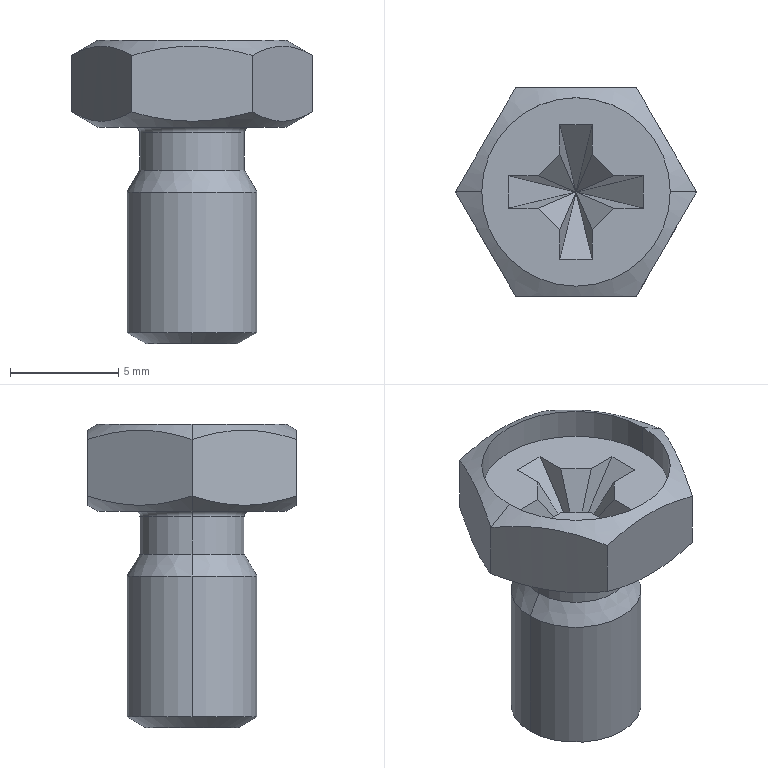Part | SolidWorks | features BaseBody 1 | 1 solid | 41 faces | box 11.131 x 9.64 x 14 mm | volume 466.025 mm3 | plane 25 | cone 8 | cylinder 6 | torus 2 | commonest cylinder face diameters 4.845 x2 6 x2 8.7 x2
STEP:
#1=CARTESIAN_POINT('',(0.,-2.134,-14.));
#2=VERTEX_POINT('',#1);
#3=CARTESIAN_POINT('',(0.,2.134,-14.));
#4=VERTEX_POINT('',#3);
#5=CARTESIAN_POINT('',(0.,0.,-14.));
#6=DIRECTION('',(0.,0.,-1.));
#7=DIRECTION('',(0.,1.,0.));
#8=AXIS2_PLACEMENT_3D('',#5,#6,#7);
#9=CIRCLE('',#8,2.134);
#10=EDGE_CURVE('',#2,#4,#9,.T.);
#11=ORIENTED_EDGE('',*,*,#10,.T.);
#12=CARTESIAN_POINT('',(0.,0.,-14.));
#13=DIRECTION('',(0.,0.,-1.));
#14=DIRECTION('',(0.,1.,0.));
#15=AXIS2_PLACEMENT_3D('',#12,#13,#14);
#16=CIRCLE('',#15,2.134);
#17=EDGE_CURVE('',#4,#2,#16,.T.);
#18=ORIENTED_EDGE('',*,*,#17,.T.);
#19=EDGE_LOOP('',(#11,#18));
#20=FACE_OUTER_BOUND('',#19,.T.);
#21=CARTESIAN_POINT('',(0.,3.,-14.));
#22=DIRECTION('',(0.,0.,1.));
#23=DIRECTION('',(1.,0.,0.));
#24=AXIS2_PLACEMENT_3D('',#21,#22,#23);
#25=PLANE('',#24);
#26=ADVANCED_FACE('',(#20),#25,.F.);
#27=CARTESIAN_POINT('',(0.,3.,-13.5));
#28=VERTEX_POINT('',#27);
#29=CARTESIAN_POINT('',(0.,3.,-13.5));
#30=DIRECTION('',(0.,0.866,0.5));
#31=VECTOR('',#30,1000.);
#32=LINE('',#29,#31);
#33=EDGE_CURVE('',#4,#28,#32,.T.);
#34=ORIENTED_EDGE('',*,*,#33,.F.);
#35=ORIENTED_EDGE('',*,*,#10,.F.);
#36=CARTESIAN_POINT('',(0.,-3.,-13.5));
#37=VERTEX_POINT('',#36);
#38=CARTESIAN_POINT('',(0.,-3.,-13.5));
#39=DIRECTION('',(0.,-0.866,0.5));
#40=VECTOR('',#39,1000.);
#41=LINE('',#38,#40);
#42=EDGE_CURVE('',#2,#37,#41,.T.);
#43=ORIENTED_EDGE('',*,*,#42,.T.);
#44=CARTESIAN_POINT('',(-3.,0.,-13.5));
#45=VERTEX_POINT('',#44);
#46=CARTESIAN_POINT('',(0.,0.,-13.5));
#47=DIRECTION('',(0.,0.,-1.));
#48=DIRECTION('',(0.,1.,0.));
#49=AXIS2_PLACEMENT_3D('',#46,#47,#48);
#50=CIRCLE('',#49,3.);
#51=EDGE_CURVE('',#37,#45,#50,.T.);
#52=ORIENTED_EDGE('',*,*,#51,.T.);
#53=CARTESIAN_POINT('',(0.,0.,-13.5));
#54=DIRECTION('',(0.,0.,-1.));
#55=DIRECTION('',(0.,1.,0.));
#56=AXIS2_PLACEMENT_3D('',#53,#54,#55);
#57=CIRCLE('',#56,3.);
#58=EDGE_CURVE('',#45,#28,#57,.T.);
#59=ORIENTED_EDGE('',*,*,#58,.T.);
#60=EDGE_LOOP('',(#34,#35,#43,#52,#59));
#61=FACE_OUTER_BOUND('',#60,.T.);
#62=CARTESIAN_POINT('',(0.,0.,-13.5));
#63=DIRECTION('',(0.,0.,1.));
#64=DIRECTION('',(0.,-1.,0.));
#65=AXIS2_PLACEMENT_3D('',#62,#63,#64);
#66=CONICAL_SURFACE('',#65,3.,1.047);
#67=ADVANCED_FACE('',(#61),#66,.T.);
#68=CARTESIAN_POINT('',(-2.673,0.,-4.));
#69=VERTEX_POINT('',#68);
#70=CARTESIAN_POINT('',(-2.423,0.,-4.25));
#71=VERTEX_POINT('',#70);
#72=CARTESIAN_POINT('',(-2.673,0.,-4.25));
#73=DIRECTION('',(0.,1.,0.));
#74=DIRECTION('',(-1.,0.,0.));
#75=AXIS2_PLACEMENT_3D('',#72,#73,#74);
#76=CIRCLE('',#75,0.25);
#77=EDGE_CURVE('',#69,#71,#76,.T.);
#78=ORIENTED_EDGE('',*,*,#77,.F.);
#79=CARTESIAN_POINT('',(2.673,0.,-4.));
#80=VERTEX_POINT('',#79);
#81=CARTESIAN_POINT('',(0.,0.,-4.));
#82=DIRECTION('',(0.,0.,1.));
#83=DIRECTION('',(1.,0.,0.));
#84=AXIS2_PLACEMENT_3D('',#81,#82,#83);
#85=CIRCLE('',#84,2.673);
#86=EDGE_CURVE('',#80,#69,#85,.T.);
#87=ORIENTED_EDGE('',*,*,#86,.F.);
#88=CARTESIAN_POINT('',(2.423,0.,-4.25));
#89=VERTEX_POINT('',#88);
#90=CARTESIAN_POINT('',(2.673,0.,-4.25));
#91=DIRECTION('',(0.,-1.,0.));
#92=DIRECTION('',(0.,0.,-1.));
#93=AXIS2_PLACEMENT_3D('',#90,#91,#92);
#94=CIRCLE('',#93,0.25);
#95=EDGE_CURVE('',#80,#89,#94,.T.);
#96=ORIENTED_EDGE('',*,*,#95,.T.);
#97=CARTESIAN_POINT('',(0.,0.,-4.25));
#98=DIRECTION('',(0.,0.,-1.));
#99=DIRECTION('',(1.,0.,0.));
#100=AXIS2_PLACEMENT_3D('',#97,#98,#99);
#101=CIRCLE('',#100,2.423);
#102=EDGE_CURVE('',#71,#89,#101,.T.);
#103=ORIENTED_EDGE('',*,*,#102,.F.);
#104=EDGE_LOOP('',(#78,#87,#96,#103));
#105=FACE_OUTER_BOUND('',#104,.T.);
#106=CARTESIAN_POINT('',(0.,0.,-4.25));
#107=DIRECTION('',(0.,0.,1.));
#108=DIRECTION('',(1.,0.,0.));
#109=AXIS2_PLACEMENT_3D('',#106,#107,#108);
#110=TOROIDAL_SURFACE('',#109,2.673,0.25);
#111=ADVANCED_FACE('',(#105),#110,.F.);
#112=CARTESIAN_POINT('',(-0.75,-1.75,-1.4));
#113=VERTEX_POINT('',#112);
#114=CARTESIAN_POINT('',(0.,0.,-4.26));
#115=VERTEX_POINT('',#114);
#116=CARTESIAN_POINT('',(-0.75,-1.75,-1.4));
#117=DIRECTION('',(0.2183,0.5093,-0.8324));
#118=VECTOR('',#117,1000.);
#119=LINE('',#116,#118);
#120=EDGE_CURVE('',#113,#115,#119,.T.);
#121=ORIENTED_EDGE('',*,*,#120,.F.);
#122=CARTESIAN_POINT('',(-0.75,-3.1,-1.4));
#123=VERTEX_POINT('',#122);
#124=CARTESIAN_POINT('',(-0.75,-1.75,-1.4));
#125=DIRECTION('',(0.,-1.,0.));
#126=VECTOR('',#125,1000.);
#127=LINE('',#124,#126);
#128=EDGE_CURVE('',#113,#123,#127,.T.);
#129=ORIENTED_EDGE('',*,*,#128,.T.);
#130=CARTESIAN_POINT('',(-0.75,-3.1,-1.4));
#131=DIRECTION('',(0.1751,0.7236,-0.6676));
#132=VECTOR('',#131,1000.);
#133=LINE('',#130,#132);
#134=EDGE_CURVE('',#123,#115,#133,.T.);
#135=ORIENTED_EDGE('',*,*,#134,.T.);
#136=EDGE_LOOP('',(#121,#129,#135));
#137=FACE_OUTER_BOUND('',#136,.T.);
#138=CARTESIAN_POINT('',(-0.75,-1.75,-1.4));
#139=DIRECTION('',(-0.9673,0.,-0.2537));
#140=DIRECTION('',(-0.2537,0.,0.9673));
#141=AXIS2_PLACEMENT_3D('',#138,#139,#140);
#142=PLANE('',#141);
#143=ADVANCED_FACE('',(#137),#142,.F.);
#144=ORIENTED_EDGE('',*,*,#134,.F.);
#145=CARTESIAN_POINT('',(0.75,-3.1,-1.4));
#146=VERTEX_POINT('',#145);
#147=CARTESIAN_POINT('',(-0.75,-3.1,-1.4));
#148=DIRECTION('',(1.,0.,0.));
#149=VECTOR('',#148,1000.);
#150=LINE('',#147,#149);
#151=EDGE_CURVE('',#123,#146,#150,.T.);
#152=ORIENTED_EDGE('',*,*,#151,.T.);
#153=CARTESIAN_POINT('',(0.75,-3.1,-1.4));
#154=DIRECTION('',(-0.1751,0.7236,-0.6676));
#155=VECTOR('',#154,1000.);
#156=LINE('',#153,#155);
#157=EDGE_CURVE('',#146,#115,#156,.T.);
#158=ORIENTED_EDGE('',*,*,#157,.T.);
#159=EDGE_LOOP('',(#144,#152,#158));
#160=FACE_OUTER_BOUND('',#159,.T.);
#161=CARTESIAN_POINT('',(-0.75,-3.1,-1.4));
#162=DIRECTION('',(0.,-0.6781,-0.735));
#163=DIRECTION('',(0.,-0.735,0.6781));
#164=AXIS2_PLACEMENT_3D('',#161,#162,#163);
#165=PLANE('',#164);
#166=ADVANCED_FACE('',(#160),#165,.F.);
#167=CARTESIAN_POINT('',(-1.75,-0.75,-1.4));
#168=VERTEX_POINT('',#167);
#169=CARTESIAN_POINT('',(-1.75,-0.75,-1.4));
#170=DIRECTION('',(0.5093,0.2183,-0.8324));
#171=VECTOR('',#170,1000.);
#172=LINE('',#169,#171);
#173=EDGE_CURVE('',#168,#115,#172,.T.);
#174=ORIENTED_EDGE('',*,*,#173,.F.);
#175=CARTESIAN_POINT('',(-1.75,-0.75,-1.4));
#176=DIRECTION('',(0.7071,-0.7071,0.));
#177=VECTOR('',#176,1000.);
#178=LINE('',#175,#177);
#179=EDGE_CURVE('',#168,#113,#178,.T.);
#180=ORIENTED_EDGE('',*,*,#179,.T.);
#181=ORIENTED_EDGE('',*,*,#120,.T.);
#182=EDGE_LOOP('',(#174,#180,#181));
#183=FACE_OUTER_BOUND('',#182,.T.);
#184=CARTESIAN_POINT('',(-1.75,-0.75,-1.4));
#185=DIRECTION('',(-0.6015,-0.6015,-0.5258));
#186=DIRECTION('',(-0.7071,0.7071,0.));
#187=AXIS2_PLACEMENT_3D('',#184,#185,#186);
#188=PLANE('',#187);
#189=ADVANCED_FACE('',(#183),#188,.F.);
#190=ORIENTED_EDGE('',*,*,#157,.F.);
#191=CARTESIAN_POINT('',(0.75,-1.75,-1.4));
#192=VERTEX_POINT('',#191);
#193=CARTESIAN_POINT('',(0.75,-1.75,-1.4));
#194=DIRECTION('',(0.,1.,0.));
#195=VECTOR('',#194,1000.);
#196=LINE('',#193,#195);
#197=EDGE_CURVE('',#146,#192,#196,.T.);
#198=ORIENTED_EDGE('',*,*,#197,.T.);
#199=CARTESIAN_POINT('',(0.75,-1.75,-1.4));
#200=DIRECTION('',(-0.2183,0.5093,-0.8324));
#201=VECTOR('',#200,1000.);
#202=LINE('',#199,#201);
#203=EDGE_CURVE('',#192,#115,#202,.T.);
#204=ORIENTED_EDGE('',*,*,#203,.T.);
#205=EDGE_LOOP('',(#190,#198,#204));
#206=FACE_OUTER_BOUND('',#205,.T.);
#207=CARTESIAN_POINT('',(0.75,-3.1,-1.4));
#208=DIRECTION('',(0.9673,0.,-0.2537));
#209=DIRECTION('',(0.,-1.,0.));
#210=AXIS2_PLACEMENT_3D('',#207,#208,#209);
#211=PLANE('',#210);
#212=ADVANCED_FACE('',(#206),#211,.F.);
#213=CARTESIAN_POINT('',(-3.1,-0.75,-1.4));
#214=VERTEX_POINT('',#213);
#215=CARTESIAN_POINT('',(-3.1,-0.75,-1.4));
#216=DIRECTION('',(0.7236,0.1751,-0.6676));
#217=VECTOR('',#216,1000.);
#218=LINE('',#215,#217);
#219=EDGE_CURVE('',#214,#115,#218,.T.);
#220=ORIENTED_EDGE('',*,*,#219,.F.);
#221=CARTESIAN_POINT('',(-3.1,-0.75,-1.4));
#222=DIRECTION('',(1.,0.,0.));
#223=VECTOR('',#222,1000.);
#224=LINE('',#221,#223);
#225=EDGE_CURVE('',#214,#168,#224,.T.);
#226=ORIENTED_EDGE('',*,*,#225,.T.);
#227=ORIENTED_EDGE('',*,*,#173,.T.);
#228=EDGE_LOOP('',(#220,#226,#227));
#229=FACE_OUTER_BOUND('',#228,.T.);
#230=CARTESIAN_POINT('',(-3.1,-0.75,-1.4));
#231=DIRECTION('',(0.,-0.9673,-0.2537));
#232=DIRECTION('',(0.,0.2537,-0.9673));
#233=AXIS2_PLACEMENT_3D('',#230,#231,#232);
#234=PLANE('',#233);
#235=ADVANCED_FACE('',(#229),#234,.F.);
#236=ORIENTED_EDGE('',*,*,#203,.F.);
#237=CARTESIAN_POINT('',(1.75,-0.75,-1.4));
#238=VERTEX_POINT('',#237);
#239=CARTESIAN_POINT('',(1.75,-0.75,-1.4));
#240=DIRECTION('',(0.7071,0.7071,0.));
#241=VECTOR('',#240,1000.);
#242=LINE('',#239,#241);
#243=EDGE_CURVE('',#192,#238,#242,.T.);
#244=ORIENTED_EDGE('',*,*,#243,.T.);
#245=CARTESIAN_POINT('',(1.75,-0.75,-1.4));
#246=DIRECTION('',(-0.5093,0.2183,-0.8324));
#247=VECTOR('',#246,1000.);
#248=LINE('',#245,#247);
#249=EDGE_CURVE('',#238,#115,#248,.T.);
#250=ORIENTED_EDGE('',*,*,#249,.T.);
#251=EDGE_LOOP('',(#236,#244,#250));
#252=FACE_OUTER_BOUND('',#251,.T.);
#253=CARTESIAN_POINT('',(0.75,-1.75,-1.4));
#254=DIRECTION('',(0.6015,-0.6015,-0.5258));
#255=DIRECTION('',(0.,0.6581,-0.7529));
#256=AXIS2_PLACEMENT_3D('',#253,#254,#255);
#257=PLANE('',#256);
#258=ADVANCED_FACE('',(#252),#257,.F.);
#259=CARTESIAN_POINT('',(-3.1,0.75,-1.4));
#260=VERTEX_POINT('',#259);
#261=CARTESIAN_POINT('',(-3.1,0.75,-1.4));
#262=DIRECTION('',(0.7236,-0.1751,-0.6676));
#263=VECTOR('',#262,1000.);
#264=LINE('',#261,#263);
#265=EDGE_CURVE('',#260,#115,#264,.T.);
#266=ORIENTED_EDGE('',*,*,#265,.F.);
#267=CARTESIAN_POINT('',(-3.1,0.75,-1.4));
#268=DIRECTION('',(0.,-1.,0.));
#269=VECTOR('',#268,1000.);
#270=LINE('',#267,#269);
#271=EDGE_CURVE('',#260,#214,#270,.T.);
#272=ORIENTED_EDGE('',*,*,#271,.T.);
#273=ORIENTED_EDGE('',*,*,#219,.T.);
#274=EDGE_LOOP('',(#266,#272,#273));
#275=FACE_OUTER_BOUND('',#274,.T.);
#276=CARTESIAN_POINT('',(-3.1,0.75,-1.4));
#277=DIRECTION('',(-0.6781,0.,-0.735));
#278=DIRECTION('',(-0.735,0.,0.6781));
#279=AXIS2_PLACEMENT_3D('',#276,#277,#278);
#280=PLANE('',#279);
#281=ADVANCED_FACE('',(#275),#280,.F.);
#282=ORIENTED_EDGE('',*,*,#249,.F.);
#283=CARTESIAN_POINT('',(3.1,-0.75,-1.4));
#284=VERTEX_POINT('',#283);
#285=CARTESIAN_POINT('',(1.75,-0.75,-1.4));
#286=DIRECTION('',(1.,0.,0.));
#287=VECTOR('',#286,1000.);
#288=LINE('',#285,#287);
#289=EDGE_CURVE('',#238,#284,#288,.T.);
#290=ORIENTED_EDGE('',*,*,#289,.T.);
#291=CARTESIAN_POINT('',(3.1,-0.75,-1.4));
#292=DIRECTION('',(-0.7236,0.1751,-0.6676));
#293=VECTOR('',#292,1000.);
#294=LINE('',#291,#293);
#295=EDGE_CURVE('',#284,#115,#294,.T.);
#296=ORIENTED_EDGE('',*,*,#295,.T.);
#297=EDGE_LOOP('',(#282,#290,#296));
#298=FACE_OUTER_BOUND('',#297,.T.);
#299=CARTESIAN_POINT('',(1.75,-0.75,-1.4));
#300=DIRECTION('',(0.,-0.9673,-0.2537));
#301=DIRECTION('',(0.,0.2537,-0.9673));
#302=AXIS2_PLACEMENT_3D('',#299,#300,#301);
#303=PLANE('',#302);
#304=ADVANCED_FACE('',(#298),#303,.F.);
#305=CARTESIAN_POINT('',(-1.75,0.75,-1.4));
#306=VERTEX_POINT('',#305);
#307=CARTESIAN_POINT('',(-1.75,0.75,-1.4));
#308=DIRECTION('',(0.5093,-0.2183,-0.8324));
#309=VECTOR('',#308,1000.);
#310=LINE('',#307,#309);
#311=EDGE_CURVE('',#306,#115,#310,.T.);
#312=ORIENTED_EDGE('',*,*,#311,.F.);
#313=CARTESIAN_POINT('',(-3.1,0.75,-1.4));
#314=DIRECTION('',(-1.,0.,0.));
#315=VECTOR('',#314,1000.);
#316=LINE('',#313,#315);
#317=EDGE_CURVE('',#306,#260,#316,.T.);
#318=ORIENTED_EDGE('',*,*,#317,.T.);
#319=ORIENTED_EDGE('',*,*,#265,.T.);
#320=EDGE_LOOP('',(#312,#318,#319));
#321=FACE_OUTER_BOUND('',#320,.T.);
#322=CARTESIAN_POINT('',(-1.75,0.75,-1.4));
#323=DIRECTION('',(0.,0.9673,-0.2537));
#324=DIRECTION('',(-1.,0.,0.));
#325=AXIS2_PLACEMENT_3D('',#322,#323,#324);
#326=PLANE('',#325);
#327=ADVANCED_FACE('',(#321),#326,.F.);
#328=ORIENTED_EDGE('',*,*,#295,.F.);
#329=CARTESIAN_POINT('',(3.1,0.75,-1.4));
#330=VERTEX_POINT('',#329);
#331=CARTESIAN_POINT('',(3.1,0.75,-1.4));
#332=DIRECTION('',(0.,1.,0.));
#333=VECTOR('',#332,1000.);
#334=LINE('',#331,#333);
#335=EDGE_CURVE('',#284,#330,#334,.T.);
#336=ORIENTED_EDGE('',*,*,#335,.T.);
#337=CARTESIAN_POINT('',(3.1,0.75,-1.4));
#338=DIRECTION('',(-0.7236,-0.1751,-0.6676));
#339=VECTOR('',#338,1000.);
#340=LINE('',#337,#339);
#341=EDGE_CURVE('',#330,#115,#340,.T.);
#342=ORIENTED_EDGE('',*,*,#341,.T.);
#343=EDGE_LOOP('',(#328,#336,#342));
#344=FACE_OUTER_BOUND('',#343,.T.);
#345=CARTESIAN_POINT('',(3.1,-0.75,-1.4));
#346=DIRECTION('',(0.6781,0.,-0.735));
#347=DIRECTION('',(0.,-1.,0.));
#348=AXIS2_PLACEMENT_3D('',#345,#346,#347);
#349=PLANE('',#348);
#350=ADVANCED_FACE('',(#344),#349,.F.);
#351=CARTESIAN_POINT('',(-0.75,1.75,-1.4));
#352=VERTEX_POINT('',#351);
#353=CARTESIAN_POINT('',(-0.75,1.75,-1.4));
#354=DIRECTION('',(0.2183,-0.5093,-0.8324));
#355=VECTOR('',#354,1000.);
#356=LINE('',#353,#355);
#357=EDGE_CURVE('',#352,#115,#356,.T.);
#358=ORIENTED_EDGE('',*,*,#357,.F.);
#359=CARTESIAN_POINT('',(-0.75,1.75,-1.4));
#360=DIRECTION('',(-0.7071,-0.7071,0.));
#361=VECTOR('',#360,1000.);
#362=LINE('',#359,#361);
#363=EDGE_CURVE('',#352,#306,#362,.T.);
#364=ORIENTED_EDGE('',*,*,#363,.T.);
#365=ORIENTED_EDGE('',*,*,#311,.T.);
#366=EDGE_LOOP('',(#358,#364,#365));
#367=FACE_OUTER_BOUND('',#366,.T.);
#368=CARTESIAN_POINT('',(-0.75,1.75,-1.4));
#369=DIRECTION('',(-0.6015,0.6015,-0.5258));
#370=DIRECTION('',(-0.6581,0.,0.7529));
#371=AXIS2_PLACEMENT_3D('',#368,#369,#370);
#372=PLANE('',#371);
#373=ADVANCED_FACE('',(#367),#372,.F.);
#374=ORIENTED_EDGE('',*,*,#341,.F.);
#375=CARTESIAN_POINT('',(1.75,0.75,-1.4));
#376=VERTEX_POINT('',#375);
#377=CARTESIAN_POINT('',(1.75,0.75,-1.4));
#378=DIRECTION('',(-1.,0.,0.));
#379=VECTOR('',#378,1000.);
#380=LINE('',#377,#379);
#381=EDGE_CURVE('',#330,#376,#380,.T.);
#382=ORIENTED_EDGE('',*,*,#381,.T.);
#383=CARTESIAN_POINT('',(1.75,0.75,-1.4));
#384=DIRECTION('',(-0.5093,-0.2183,-0.8324));
#385=VECTOR('',#384,1000.);
#386=LINE('',#383,#385);
#387=EDGE_CURVE('',#376,#115,#386,.T.);
#388=ORIENTED_EDGE('',*,*,#387,.T.);
#389=EDGE_LOOP('',(#374,#382,#388));
#390=FACE_OUTER_BOUND('',#389,.T.);
#391=CARTESIAN_POINT('',(3.1,0.75,-1.4));
#392=DIRECTION('',(0.,0.9673,-0.2537));
#393=DIRECTION('',(-1.,0.,0.));
#394=AXIS2_PLACEMENT_3D('',#391,#392,#393);
#395=PLANE('',#394);
#396=ADVANCED_FACE('',(#390),#395,.F.);
#397=CARTESIAN_POINT('',(-0.75,3.1,-1.4));
#398=VERTEX_POINT('',#397);
#399=CARTESIAN_POINT('',(-0.75,3.1,-1.4));
#400=DIRECTION('',(0.1751,-0.7236,-0.6676));
#401=VECTOR('',#400,1000.);
#402=LINE('',#399,#401);
#403=EDGE_CURVE('',#398,#115,#402,.T.);
#404=ORIENTED_EDGE('',*,*,#403,.F.);
#405=CARTESIAN_POINT('',(-0.75,3.1,-1.4));
#406=DIRECTION('',(0.,-1.,0.));
#407=VECTOR('',#406,1000.);
#408=LINE('',#405,#407);
#409=EDGE_CURVE('',#398,#352,#408,.T.);
#410=ORIENTED_EDGE('',*,*,#409,.T.);
#411=ORIENTED_EDGE('',*,*,#357,.T.);
#412=EDGE_LOOP('',(#404,#410,#411));
#413=FACE_OUTER_BOUND('',#412,.T.);
#414=CARTESIAN_POINT('',(-0.75,3.1,-1.4));
#415=DIRECTION('',(-0.9673,0.,-0.2537));
#416=DIRECTION('',(-0.2537,0.,0.9673));
#417=AXIS2_PLACEMENT_3D('',#414,#415,#416);
#418=PLANE('',#417);
#419=ADVANCED_FACE('',(#413),#418,.F.);
#420=ORIENTED_EDGE('',*,*,#387,.F.);
#421=CARTESIAN_POINT('',(0.75,1.75,-1.4));
#422=VERTEX_POINT('',#421);
#423=CARTESIAN_POINT('',(0.75,1.75,-1.4));
#424=DIRECTION('',(-0.7071,0.7071,0.));
#425=VECTOR('',#424,1000.);
#426=LINE('',#423,#425);
#427=EDGE_CURVE('',#376,#422,#426,.T.);
#428=ORIENTED_EDGE('',*,*,#427,.T.);
#429=CARTESIAN_POINT('',(0.75,1.75,-1.4));
#430=DIRECTION('',(-0.2183,-0.5093,-0.8324));
#431=VECTOR('',#430,1000.);
#432=LINE('',#429,#431);
#433=EDGE_CURVE('',#422,#115,#432,.T.);
#434=ORIENTED_EDGE('',*,*,#433,.T.);
#435=EDGE_LOOP('',(#420,#428,#434));
#436=FACE_OUTER_BOUND('',#435,.T.);
#437=CARTESIAN_POINT('',(1.75,0.75,-1.4));
#438=DIRECTION('',(0.6015,0.6015,-0.5258));
#439=DIRECTION('',(0.,-0.6581,-0.7529));
#440=AXIS2_PLACEMENT_3D('',#437,#438,#439);
#441=PLANE('',#440);
#442=ADVANCED_FACE('',(#436),#441,.F.);
#443=CARTESIAN_POINT('',(0.75,3.1,-1.4));
#444=VERTEX_POINT('',#443);
#445=CARTESIAN_POINT('',(0.75,3.1,-1.4));
#446=DIRECTION('',(-0.1751,-0.7236,-0.6676));
#447=VECTOR('',#446,1000.);
#448=LINE('',#445,#447);
#449=EDGE_CURVE('',#444,#115,#448,.T.);
#450=ORIENTED_EDGE('',*,*,#449,.F.);
#451=CARTESIAN_POINT('',(-0.75,3.1,-1.4));
#452=DIRECTION('',(-1.,0.,0.));
#453=VECTOR('',#452,1000.);
#454=LINE('',#451,#453);
#455=EDGE_CURVE('',#444,#398,#454,.T.);
#456=ORIENTED_EDGE('',*,*,#455,.T.);
#457=ORIENTED_EDGE('',*,*,#403,.T.);
#458=EDGE_LOOP('',(#450,#456,#457));
#459=FACE_OUTER_BOUND('',#458,.T.);
#460=CARTESIAN_POINT('',(0.75,3.1,-1.4));
#461=DIRECTION('',(0.,0.6781,-0.735));
#462=DIRECTION('',(-1.,0.,0.));
#463=AXIS2_PLACEMENT_3D('',#460,#461,#462);
#464=PLANE('',#463);
#465=ADVANCED_FACE('',(#459),#464,.F.);
#466=ORIENTED_EDGE('',*,*,#433,.F.);
#467=CARTESIAN_POINT('',(0.75,3.1,-1.4));
#468=DIRECTION('',(0.,1.,0.));
#469=VECTOR('',#468,1000.);
#470=LINE('',#467,#469);
#471=EDGE_CURVE('',#422,#444,#470,.T.);
#472=ORIENTED_EDGE('',*,*,#471,.T.);
#473=ORIENTED_EDGE('',*,*,#449,.T.);
#474=EDGE_LOOP('',(#466,#472,#473));
#475=FACE_OUTER_BOUND('',#474,.T.);
#476=CARTESIAN_POINT('',(0.75,1.75,-1.4));
#477=DIRECTION('',(0.9673,0.,-0.2537));
#478=DIRECTION('',(0.,-1.,0.));
#479=AXIS2_PLACEMENT_3D('',#476,#477,#478);
#480=PLANE('',#479);
#481=ADVANCED_FACE('',(#475),#480,.F.);
#482=ORIENTED_EDGE('',*,*,#471,.F.);
#483=ORIENTED_EDGE('',*,*,#427,.F.);
#484=ORIENTED_EDGE('',*,*,#381,.F.);
#485=ORIENTED_EDGE('',*,*,#335,.F.);
#486=ORIENTED_EDGE('',*,*,#289,.F.);
#487=ORIENTED_EDGE('',*,*,#243,.F.);
#488=ORIENTED_EDGE('',*,*,#197,.F.);
#489=ORIENTED_EDGE('',*,*,#151,.F.);
#490=ORIENTED_EDGE('',*,*,#128,.F.);
#491=ORIENTED_EDGE('',*,*,#179,.F.);
#492=ORIENTED_EDGE('',*,*,#225,.F.);
#493=ORIENTED_EDGE('',*,*,#271,.F.);
#494=ORIENTED_EDGE('',*,*,#317,.F.);
#495=ORIENTED_EDGE('',*,*,#363,.F.);
#496=ORIENTED_EDGE('',*,*,#409,.F.);
#497=ORIENTED_EDGE('',*,*,#455,.F.);
#498=EDGE_LOOP('',(#482,#483,#484,#485,#486,#487,#488,#489,#490,#491,#492,#493,#494,#495,#496,#497));
#499=FACE_BOUND('',#498,.T.);
#500=CARTESIAN_POINT('',(4.35,0.,-1.4));
#501=VERTEX_POINT('',#500);
#502=CARTESIAN_POINT('',(-4.35,0.,-1.4));
#503=VERTEX_POINT('',#502);
#504=CARTESIAN_POINT('',(0.,0.,-1.4));
#505=DIRECTION('',(0.,0.,1.));
#506=DIRECTION('',(1.,0.,0.));
#507=AXIS2_PLACEMENT_3D('',#504,#505,#506);
#508=CIRCLE('',#507,4.35);
#509=EDGE_CURVE('',#501,#503,#508,.T.);
#510=ORIENTED_EDGE('',*,*,#509,.T.);
#511=CARTESIAN_POINT('',(0.,0.,-1.4));
#512=DIRECTION('',(0.,0.,1.));
#513=DIRECTION('',(1.,0.,0.));
#514=AXIS2_PLACEMENT_3D('',#511,#512,#513);
#515=CIRCLE('',#514,4.35);
#516=EDGE_CURVE('',#503,#501,#515,.T.);
#517=ORIENTED_EDGE('',*,*,#516,.T.);
#518=EDGE_LOOP('',(#510,#517));
#519=FACE_OUTER_BOUND('',#518,.T.);
#520=CARTESIAN_POINT('',(0.,0.,-1.4));
#521=DIRECTION('',(0.,0.,1.));
#522=DIRECTION('',(1.,0.,0.));
#523=AXIS2_PLACEMENT_3D('',#520,#521,#522);
#524=PLANE('',#523);
#525=ADVANCED_FACE('',(#499,#519),#524,.T.);
#526=CARTESIAN_POINT('',(-4.35,0.,0.));
#527=VERTEX_POINT('',#526);
#528=CARTESIAN_POINT('',(-4.35,0.,-1.4));
#529=DIRECTION('',(0.,0.,1.));
#530=VECTOR('',#529,1000.);
#531=LINE('',#528,#530);
#532=EDGE_CURVE('',#503,#527,#531,.T.);
#533=ORIENTED_EDGE('',*,*,#532,.F.);
#534=ORIENTED_EDGE('',*,*,#509,.F.);
#535=CARTESIAN_POINT('',(4.35,0.,0.));
#536=VERTEX_POINT('',#535);
#537=CARTESIAN_POINT('',(4.35,0.,-1.4));
#538=DIRECTION('',(0.,0.,1.));
#539=VECTOR('',#538,1000.);
#540=LINE('',#537,#539);
#541=EDGE_CURVE('',#501,#536,#540,.T.);
#542=ORIENTED_EDGE('',*,*,#541,.T.);
#543=CARTESIAN_POINT('',(0.,0.,0.));
#544=DIRECTION('',(0.,0.,1.));
#545=DIRECTION('',(1.,0.,0.));
#546=AXIS2_PLACEMENT_3D('',#543,#544,#545);
#547=CIRCLE('',#546,4.35);
#548=EDGE_CURVE('',#536,#527,#547,.T.);
#549=ORIENTED_EDGE('',*,*,#548,.T.);
#550=EDGE_LOOP('',(#533,#534,#542,#549));
#551=FACE_OUTER_BOUND('',#550,.T.);
#552=CARTESIAN_POINT('',(0.,0.,-1.4));
#553=DIRECTION('',(0.,0.,1.));
#554=DIRECTION('',(1.,0.,0.));
#555=AXIS2_PLACEMENT_3D('',#552,#553,#554);
#556=CYLINDRICAL_SURFACE('',#555,4.35);
#557=ADVANCED_FACE('',(#551),#556,.F.);
#558=CARTESIAN_POINT('',(5.566,0.,-0.7019));
#559=VERTEX_POINT('',#558);
#560=CARTESIAN_POINT('',(4.35,0.,0.));
#561=DIRECTION('',(0.866,0.,-0.5));
#562=VECTOR('',#561,1000.);
#563=LINE('',#560,#562);
#564=EDGE_CURVE('',#536,#559,#563,.T.);
#565=ORIENTED_EDGE('',*,*,#564,.F.);
#566=CARTESIAN_POINT('',(0.,0.,0.));
#567=DIRECTION('',(0.,0.,1.));
#568=DIRECTION('',(1.,0.,0.));
#569=AXIS2_PLACEMENT_3D('',#566,#567,#568);
#570=CIRCLE('',#569,4.35);
#571=EDGE_CURVE('',#527,#536,#570,.T.);
#572=ORIENTED_EDGE('',*,*,#571,.F.);
#573=CARTESIAN_POINT('',(-5.566,0.,-0.7019));
#574=VERTEX_POINT('',#573);
#575=CARTESIAN_POINT('',(-4.35,0.,0.));
#576=DIRECTION('',(-0.866,0.,-0.5));
#577=VECTOR('',#576,1000.);
#578=LINE('',#575,#577);
#579=EDGE_CURVE('',#527,#574,#578,.T.);
#580=ORIENTED_EDGE('',*,*,#579,.T.);
#581=CARTESIAN_POINT('',(-2.783,-4.82,-0.7019));
#582=VERTEX_POINT('',#581);
#583=CARTESIAN_POINT('',(-5.566,0.,-0.7019));
#584=CARTESIAN_POINT('',(-5.447,-0.2048,-0.6336));
#585=CARTESIAN_POINT('',(-5.332,-0.4051,-0.5733));
#586=CARTESIAN_POINT('',(-5.161,-0.7017,-0.4948));
#587=CARTESIAN_POINT('',(-5.104,-0.7999,-0.4706));
#588=CARTESIAN_POINT('',(-5.019,-0.9467,-0.4374));
#589=CARTESIAN_POINT('',(-4.977,-1.02,-0.4215));
#590=CARTESIAN_POINT('',(-4.935,-1.093,-0.4067));
#591=CARTESIAN_POINT('',(-4.907,-1.142,-0.3971));
#592=CARTESIAN_POINT('',(-4.894,-1.165,-0.3927));
#593=CARTESIAN_POINT('',(-4.759,-1.398,-0.3492));
#594=CARTESIAN_POINT('',(-4.642,-1.6,-0.3201));
#595=CARTESIAN_POINT('',(-4.41,-2.002,-0.2813));
#596=CARTESIAN_POINT('',(-4.295,-2.201,-0.2715));
#597=CARTESIAN_POINT('',(-4.059,-2.61,-0.2712));
#598=CARTESIAN_POINT('',(-3.942,-2.811,-0.2808));
#599=CARTESIAN_POINT('',(-3.767,-3.115,-0.3097));
#600=CARTESIAN_POINT('',(-3.709,-3.216,-0.3218));
#601=CARTESIAN_POINT('',(-3.62,-3.369,-0.3436));
#602=CARTESIAN_POINT('',(-3.576,-3.446,-0.3554));
#603=CARTESIAN_POINT('',(-3.532,-3.523,-0.3685));
#604=CARTESIAN_POINT('',(-3.502,-3.575,-0.3776));
#605=CARTESIAN_POINT('',(-3.486,-3.602,-0.3826));
#606=CARTESIAN_POINT('',(-3.247,-4.017,-0.4599));
#607=CARTESIAN_POINT('',(-3.02,-4.409,-0.5648));
#608=CARTESIAN_POINT('',(-2.783,-4.82,-0.7019));
#609=B_SPLINE_CURVE_WITH_KNOTS('',3,(#583,#584,#585,#586,#587,#588,#589,#590,#591,#592,#593,#594,#595,#596,#597,#598,#599,#600,#601,#602,#603,#604,#605,#606,#607,#608),.UNSPECIFIED.,.F.,.F.,(4,2,2,1,2,2,2,2,2,2,1,2,2,4),(0.,0.125,0.1875,0.2187,0.2344,0.25,0.375,0.5,0.625,0.6875,0.7188,0.7344,0.75,1.),.UNSPECIFIED.);
#610=EDGE_CURVE('',#574,#582,#609,.T.);
#611=ORIENTED_EDGE('',*,*,#610,.T.);
#612=CARTESIAN_POINT('',(2.783,-4.82,-0.7019));
#613=VERTEX_POINT('',#612);
#614=CARTESIAN_POINT('',(-2.783,-4.82,-0.7019));
#615=CARTESIAN_POINT('',(-2.545,-4.82,-0.6332));
#616=CARTESIAN_POINT('',(-2.312,-4.82,-0.5726));
#617=CARTESIAN_POINT('',(-1.968,-4.82,-0.4938));
#618=CARTESIAN_POINT('',(-1.854,-4.82,-0.4695));
#619=CARTESIAN_POINT('',(-1.684,-4.82,-0.4362));
#620=CARTESIAN_POINT('',(-1.599,-4.82,-0.4202));
#621=CARTESIAN_POINT('',(-1.515,-4.82,-0.4055));
#622=CARTESIAN_POINT('',(-1.458,-4.82,-0.3959));
#623=CARTESIAN_POINT('',(-1.431,-4.82,-0.3914));
#624=CARTESIAN_POINT('',(-0.9247,-4.82,-0.3097));
#625=CARTESIAN_POINT('',(-0.4706,-4.82,-0.2713));
#626=CARTESIAN_POINT('',(0.1187,-4.82,-0.2714));
#627=CARTESIAN_POINT('',(0.2362,-4.82,-0.2739));
#628=CARTESIAN_POINT('',(0.4717,-4.82,-0.2839));
#629=CARTESIAN_POINT('',(0.5915,-4.82,-0.2915));
#630=CARTESIAN_POINT('',(0.826,-4.82,-0.3112));
#631=CARTESIAN_POINT('',(0.9429,-4.82,-0.3234));
#632=CARTESIAN_POINT('',(1.119,-4.82,-0.3451));
#633=CARTESIAN_POINT('',(1.206,-4.82,-0.3569));
#634=CARTESIAN_POINT('',(1.295,-4.82,-0.3699));
#635=CARTESIAN_POINT('',(1.354,-4.82,-0.3789));
#636=CARTESIAN_POINT('',(1.385,-4.82,-0.3838));
#637=CARTESIAN_POINT('',(1.86,-4.82,-0.4611));
#638=CARTESIAN_POINT('',(2.311,-4.82,-0.5656));
#639=CARTESIAN_POINT('',(2.783,-4.82,-0.7019));
#640=B_SPLINE_CURVE_WITH_KNOTS('',3,(#614,#615,#616,#617,#618,#619,#620,#621,#622,#623,#624,#625,#626,#627,#628,#629,#630,#631,#632,#633,#634,#635,#636,#637,#638,#639),.UNSPECIFIED.,.F.,.F.,(4,2,2,1,2,2,2,2,2,2,1,2,2,4),(0.,0.125,0.1875,0.2188,0.2344,0.25,0.5,0.5625,0.625,0.6875,0.7188,0.7344,0.75,1.),.UNSPECIFIED.);
#641=EDGE_CURVE('',#582,#613,#640,.T.);
#642=ORIENTED_EDGE('',*,*,#641,.T.);
#643=CARTESIAN_POINT('',(2.783,-4.82,-0.7019));
#644=CARTESIAN_POINT('',(2.901,-4.615,-0.6336));
#645=CARTESIAN_POINT('',(3.017,-4.415,-0.5733));
#646=CARTESIAN_POINT('',(3.188,-4.118,-0.4948));
#647=CARTESIAN_POINT('',(3.245,-4.02,-0.4706));
#648=CARTESIAN_POINT('',(3.33,-3.873,-0.4374));
#649=CARTESIAN_POINT('',(3.372,-3.8,-0.4215));
#650=CARTESIAN_POINT('',(3.414,-3.727,-0.4067));
#651=CARTESIAN_POINT('',(3.442,-3.678,-0.3971));
#652=CARTESIAN_POINT('',(3.455,-3.656,-0.3927));
#653=CARTESIAN_POINT('',(3.59,-3.423,-0.3492));
#654=CARTESIAN_POINT('',(3.706,-3.22,-0.3201));
#655=CARTESIAN_POINT('',(3.938,-2.818,-0.2813));
#656=CARTESIAN_POINT('',(4.053,-2.619,-0.2715));
#657=CARTESIAN_POINT('',(4.29,-2.21,-0.2712));
#658=CARTESIAN_POINT('',(4.406,-2.008,-0.2808));
#659=CARTESIAN_POINT('',(4.581,-1.705,-0.3097));
#660=CARTESIAN_POINT('',(4.639,-1.604,-0.3218));
#661=CARTESIAN_POINT('',(4.728,-1.451,-0.3436));
#662=CARTESIAN_POINT('',(4.772,-1.374,-0.3554));
#663=CARTESIAN_POINT('',(4.817,-1.297,-0.3685));
#664=CARTESIAN_POINT('',(4.847,-1.245,-0.3776));
#665=CARTESIAN_POINT('',(4.863,-1.218,-0.3826));
#666=CARTESIAN_POINT('',(5.102,-0.8033,-0.4599));
#667=CARTESIAN_POINT('',(5.328,-0.4112,-0.5648));
#668=CARTESIAN_POINT('',(5.566,0.,-0.7019));
#669=B_SPLINE_CURVE_WITH_KNOTS('',3,(#643,#644,#645,#646,#647,#648,#649,#650,#651,#652,#653,#654,#655,#656,#657,#658,#659,#660,#661,#662,#663,#664,#665,#666,#667,#668),.UNSPECIFIED.,.F.,.F.,(4,2,2,1,2,2,2,2,2,2,1,2,2,4),(0.,0.125,0.1875,0.2187,0.2344,0.25,0.375,0.5,0.625,0.6875,0.7187,0.7344,0.75,1.),.UNSPECIFIED.);
#670=EDGE_CURVE('',#613,#559,#669,.T.);
#671=ORIENTED_EDGE('',*,*,#670,.T.);
#672=EDGE_LOOP('',(#565,#572,#580,#611,#642,#671));
#673=FACE_OUTER_BOUND('',#672,.T.);
#674=CARTESIAN_POINT('',(0.,0.,0.));
#675=DIRECTION('',(0.,0.,-1.));
#676=DIRECTION('',(-1.,0.,0.));
#677=AXIS2_PLACEMENT_3D('',#674,#675,#676);
#678=CONICAL_SURFACE('',#677,4.35,1.047);
#679=ADVANCED_FACE('',(#673),#678,.T.);
#680=ORIENTED_EDGE('',*,*,#670,.F.);
#681=CARTESIAN_POINT('',(2.783,-4.82,-3.298));
#682=VERTEX_POINT('',#681);
#683=CARTESIAN_POINT('',(2.783,-4.82,-4.));
#684=DIRECTION('',(0.,0.,1.));
#685=VECTOR('',#684,1000.);
#686=LINE('',#683,#685);
#687=EDGE_CURVE('',#682,#613,#686,.T.);
#688=ORIENTED_EDGE('',*,*,#687,.F.);
#689=CARTESIAN_POINT('',(5.566,0.,-3.298));
#690=VERTEX_POINT('',#689);
#691=CARTESIAN_POINT('',(5.566,0.,-3.298));
#692=CARTESIAN_POINT('',(5.447,-0.2048,-3.366));
#693=CARTESIAN_POINT('',(5.332,-0.4051,-3.427));
#694=CARTESIAN_POINT('',(5.161,-0.7017,-3.505));
#695=CARTESIAN_POINT('',(5.104,-0.7999,-3.529));
#696=CARTESIAN_POINT('',(5.019,-0.9467,-3.563));
#697=CARTESIAN_POINT('',(4.977,-1.02,-3.579));
#698=CARTESIAN_POINT('',(4.935,-1.093,-3.593));
#699=CARTESIAN_POINT('',(4.907,-1.142,-3.603));
#700=CARTESIAN_POINT('',(4.894,-1.165,-3.607));
#701=CARTESIAN_POINT('',(4.759,-1.398,-3.651));
#702=CARTESIAN_POINT('',(4.642,-1.6,-3.68));
#703=CARTESIAN_POINT('',(4.41,-2.002,-3.719));
#704=CARTESIAN_POINT('',(4.295,-2.201,-3.728));
#705=CARTESIAN_POINT('',(4.059,-2.61,-3.729));
#706=CARTESIAN_POINT('',(3.942,-2.811,-3.719));
#707=CARTESIAN_POINT('',(3.767,-3.115,-3.69));
#708=CARTESIAN_POINT('',(3.709,-3.216,-3.678));
#709=CARTESIAN_POINT('',(3.62,-3.369,-3.656));
#710=CARTESIAN_POINT('',(3.576,-3.446,-3.645));
#711=CARTESIAN_POINT('',(3.532,-3.523,-3.631));
#712=CARTESIAN_POINT('',(3.502,-3.575,-3.622));
#713=CARTESIAN_POINT('',(3.486,-3.602,-3.617));
#714=CARTESIAN_POINT('',(3.247,-4.017,-3.54));
#715=CARTESIAN_POINT('',(3.02,-4.409,-3.435));
#716=CARTESIAN_POINT('',(2.783,-4.82,-3.298));
#717=B_SPLINE_CURVE_WITH_KNOTS('',3,(#691,#692,#693,#694,#695,#696,#697,#698,#699,#700,#701,#702,#703,#704,#705,#706,#707,#708,#709,#710,#711,#712,#713,#714,#715,#716),.UNSPECIFIED.,.F.,.F.,(4,2,2,1,2,2,2,2,2,2,1,2,2,4),(0.,0.125,0.1875,0.2187,0.2344,0.25,0.375,0.5,0.625,0.6875,0.7187,0.7344,0.75,1.),.UNSPECIFIED.);
#718=EDGE_CURVE('',#690,#682,#717,.T.);
#719=ORIENTED_EDGE('',*,*,#718,.F.);
#720=CARTESIAN_POINT('',(5.566,0.,-4.));
#721=DIRECTION('',(0.,0.,1.));
#722=VECTOR('',#721,1000.);
#723=LINE('',#720,#722);
#724=EDGE_CURVE('',#690,#559,#723,.T.);
#725=ORIENTED_EDGE('',*,*,#724,.T.);
#726=EDGE_LOOP('',(#680,#688,#719,#725));
#727=FACE_OUTER_BOUND('',#726,.T.);
#728=CARTESIAN_POINT('',(2.783,-4.82,-4.));
#729=DIRECTION('',(0.866,-0.5,0.));
#730=DIRECTION('',(0.,0.,-1.));
#731=AXIS2_PLACEMENT_3D('',#728,#729,#730);
#732=PLANE('',#731);
#733=ADVANCED_FACE('',(#727),#732,.T.);
#734=ORIENTED_EDGE('',*,*,#641,.F.);
#735=CARTESIAN_POINT('',(-2.783,-4.82,-3.298));
#736=VERTEX_POINT('',#735);
#737=CARTESIAN_POINT('',(-2.783,-4.82,-4.));
#738=DIRECTION('',(0.,0.,1.));
#739=VECTOR('',#738,1000.);
#740=LINE('',#737,#739);
#741=EDGE_CURVE('',#736,#582,#740,.T.);
#742=ORIENTED_EDGE('',*,*,#741,.F.);
#743=CARTESIAN_POINT('',(2.783,-4.82,-3.298));
#744=CARTESIAN_POINT('',(2.547,-4.82,-3.366));
#745=CARTESIAN_POINT('',(2.316,-4.82,-3.426));
#746=CARTESIAN_POINT('',(1.975,-4.82,-3.505));
#747=CARTESIAN_POINT('',(1.862,-4.82,-3.529));
#748=CARTESIAN_POINT('',(1.693,-4.82,-3.562));
#749=CARTESIAN_POINT('',(1.609,-4.82,-3.578));
#750=CARTESIAN_POINT('',(1.525,-4.82,-3.593));
#751=CARTESIAN_POINT('',(1.468,-4.82,-3.602));
#752=CARTESIAN_POINT('',(1.442,-4.82,-3.607));
#753=CARTESIAN_POINT('',(1.294,-4.82,-3.631));
#754=CARTESIAN_POINT('',(1.177,-4.82,-3.648));
#755=CARTESIAN_POINT('',(0.9429,-4.82,-3.677));
#756=CARTESIAN_POINT('',(0.8277,-4.82,-3.689));
#757=CARTESIAN_POINT('',(0.4709,-4.82,-3.719));
#758=CARTESIAN_POINT('',(0.2358,-4.82,-3.729));
#759=CARTESIAN_POINT('',(-0.2342,-4.82,-3.729));
#760=CARTESIAN_POINT('',(-0.4655,-4.82,-3.719));
#761=CARTESIAN_POINT('',(-0.8138,-4.82,-3.69));
#762=CARTESIAN_POINT('',(-0.9302,-4.82,-3.678));
#763=CARTESIAN_POINT('',(-1.106,-4.82,-3.657));
#764=CARTESIAN_POINT('',(-1.194,-4.82,-3.645));
#765=CARTESIAN_POINT('',(-1.283,-4.82,-3.632));
#766=CARTESIAN_POINT('',(-1.342,-4.82,-3.623));
#767=CARTESIAN_POINT('',(-1.373,-4.82,-3.618));
#768=CARTESIAN_POINT('',(-1.853,-4.82,-3.541));
#769=CARTESIAN_POINT('',(-2.307,-4.82,-3.436));
#770=CARTESIAN_POINT('',(-2.783,-4.82,-3.298));
#771=B_SPLINE_CURVE_WITH_KNOTS('',3,(#743,#744,#745,#746,#747,#748,#749,#750,#751,#752,#753,#754,#755,#756,#757,#758,#759,#760,#761,#762,#763,#764,#765,#766,#767,#768,#769,#770),.UNSPECIFIED.,.F.,.F.,(4,2,2,1,2,2,2,2,2,2,2,1,2,2,4),(0.,0.125,0.1875,0.2188,0.2344,0.25,0.3125,0.375,0.5,0.625,0.6875,0.7188,0.7344,0.75,1.),.UNSPECIFIED.);
#772=EDGE_CURVE('',#682,#736,#771,.T.);
#773=ORIENTED_EDGE('',*,*,#772,.F.);
#774=ORIENTED_EDGE('',*,*,#687,.T.);
#775=EDGE_LOOP('',(#734,#742,#773,#774));
#776=FACE_OUTER_BOUND('',#775,.T.);
#777=CARTESIAN_POINT('',(-2.783,-4.82,-4.));
#778=DIRECTION('',(0.,-1.,0.));
#779=DIRECTION('',(-1.,0.,0.));
#780=AXIS2_PLACEMENT_3D('',#777,#778,#779);
#781=PLANE('',#780);
#782=ADVANCED_FACE('',(#776),#781,.T.);
#783=ORIENTED_EDGE('',*,*,#610,.F.);
#784=CARTESIAN_POINT('',(-5.566,0.,-3.298));
#785=VERTEX_POINT('',#784);
#786=CARTESIAN_POINT('',(-5.566,0.,-4.));
#787=DIRECTION('',(0.,0.,1.));
#788=VECTOR('',#787,1000.);
#789=LINE('',#786,#788);
#790=EDGE_CURVE('',#785,#574,#789,.T.);
#791=ORIENTED_EDGE('',*,*,#790,.F.);
#792=CARTESIAN_POINT('',(-2.783,-4.82,-3.298));
#793=CARTESIAN_POINT('',(-2.901,-4.615,-3.366));
#794=CARTESIAN_POINT('',(-3.017,-4.415,-3.427));
#795=CARTESIAN_POINT('',(-3.188,-4.118,-3.505));
#796=CARTESIAN_POINT('',(-3.245,-4.02,-3.529));
#797=CARTESIAN_POINT('',(-3.33,-3.873,-3.563));
#798=CARTESIAN_POINT('',(-3.372,-3.8,-3.579));
#799=CARTESIAN_POINT('',(-3.414,-3.727,-3.593));
#800=CARTESIAN_POINT('',(-3.442,-3.678,-3.603));
#801=CARTESIAN_POINT('',(-3.455,-3.656,-3.607));
#802=CARTESIAN_POINT('',(-3.59,-3.423,-3.651));
#803=CARTESIAN_POINT('',(-3.706,-3.22,-3.68));
#804=CARTESIAN_POINT('',(-3.938,-2.818,-3.719));
#805=CARTESIAN_POINT('',(-4.053,-2.619,-3.728));
#806=CARTESIAN_POINT('',(-4.29,-2.21,-3.729));
#807=CARTESIAN_POINT('',(-4.406,-2.008,-3.719));
#808=CARTESIAN_POINT('',(-4.581,-1.705,-3.69));
#809=CARTESIAN_POINT('',(-4.639,-1.604,-3.678));
#810=CARTESIAN_POINT('',(-4.728,-1.451,-3.656));
#811=CARTESIAN_POINT('',(-4.772,-1.374,-3.645));
#812=CARTESIAN_POINT('',(-4.817,-1.297,-3.631));
#813=CARTESIAN_POINT('',(-4.847,-1.245,-3.622));
#814=CARTESIAN_POINT('',(-4.863,-1.218,-3.617));
#815=CARTESIAN_POINT('',(-5.102,-0.8033,-3.54));
#816=CARTESIAN_POINT('',(-5.328,-0.4112,-3.435));
#817=CARTESIAN_POINT('',(-5.566,0.,-3.298));
#818=B_SPLINE_CURVE_WITH_KNOTS('',3,(#792,#793,#794,#795,#796,#797,#798,#799,#800,#801,#802,#803,#804,#805,#806,#807,#808,#809,#810,#811,#812,#813,#814,#815,#816,#817),.UNSPECIFIED.,.F.,.F.,(4,2,2,1,2,2,2,2,2,2,1,2,2,4),(0.,0.125,0.1875,0.2188,0.2344,0.25,0.375,0.5,0.625,0.6875,0.7188,0.7344,0.75,1.),.UNSPECIFIED.);
#819=EDGE_CURVE('',#736,#785,#818,.T.);
#820=ORIENTED_EDGE('',*,*,#819,.F.);
#821=ORIENTED_EDGE('',*,*,#741,.T.);
#822=EDGE_LOOP('',(#783,#791,#820,#821));
#823=FACE_OUTER_BOUND('',#822,.T.);
#824=CARTESIAN_POINT('',(-5.566,0.,-4.));
#825=DIRECTION('',(-0.866,-0.5,0.));
#826=DIRECTION('',(-0.5,0.866,0.));
#827=AXIS2_PLACEMENT_3D('',#824,#825,#826);
#828=PLANE('',#827);
#829=ADVANCED_FACE('',(#823),#828,.T.);
#830=CARTESIAN_POINT('',(-2.783,4.82,-0.7019));
#831=VERTEX_POINT('',#830);
#832=CARTESIAN_POINT('',(-2.783,4.82,-0.7019));
#833=CARTESIAN_POINT('',(-2.901,4.615,-0.6336));
#834=CARTESIAN_POINT('',(-3.017,4.415,-0.5733));
#835=CARTESIAN_POINT('',(-3.188,4.118,-0.4948));
#836=CARTESIAN_POINT('',(-3.245,4.02,-0.4706));
#837=CARTESIAN_POINT('',(-3.33,3.873,-0.4374));
#838=CARTESIAN_POINT('',(-3.372,3.8,-0.4215));
#839=CARTESIAN_POINT('',(-3.414,3.727,-0.4067));
#840=CARTESIAN_POINT('',(-3.442,3.678,-0.3971));
#841=CARTESIAN_POINT('',(-3.455,3.656,-0.3927));
#842=CARTESIAN_POINT('',(-3.59,3.423,-0.3492));
#843=CARTESIAN_POINT('',(-3.706,3.22,-0.3201));
#844=CARTESIAN_POINT('',(-3.938,2.818,-0.2813));
#845=CARTESIAN_POINT('',(-4.053,2.619,-0.2715));
#846=CARTESIAN_POINT('',(-4.29,2.21,-0.2712));
#847=CARTESIAN_POINT('',(-4.406,2.008,-0.2808));
#848=CARTESIAN_POINT('',(-4.581,1.705,-0.3097));
#849=CARTESIAN_POINT('',(-4.639,1.604,-0.3218));
#850=CARTESIAN_POINT('',(-4.728,1.451,-0.3436));
#851=CARTESIAN_POINT('',(-4.772,1.374,-0.3554));
#852=CARTESIAN_POINT('',(-4.817,1.297,-0.3685));
#853=CARTESIAN_POINT('',(-4.847,1.245,-0.3776));
#854=CARTESIAN_POINT('',(-4.863,1.218,-0.3826));
#855=CARTESIAN_POINT('',(-5.102,0.8033,-0.4599));
#856=CARTESIAN_POINT('',(-5.328,0.4112,-0.5648));
#857=CARTESIAN_POINT('',(-5.566,0.,-0.7019));
#858=B_SPLINE_CURVE_WITH_KNOTS('',3,(#832,#833,#834,#835,#836,#837,#838,#839,#840,#841,#842,#843,#844,#845,#846,#847,#848,#849,#850,#851,#852,#853,#854,#855,#856,#857),.UNSPECIFIED.,.F.,.F.,(4,2,2,1,2,2,2,2,2,2,1,2,2,4),(0.,0.125,0.1875,0.2188,0.2344,0.25,0.375,0.5,0.625,0.6875,0.7187,0.7344,0.75,1.),.UNSPECIFIED.);
#859=EDGE_CURVE('',#831,#574,#858,.T.);
#860=ORIENTED_EDGE('',*,*,#859,.F.);
#861=CARTESIAN_POINT('',(-2.783,4.82,-3.298));
#862=VERTEX_POINT('',#861);
#863=CARTESIAN_POINT('',(-2.783,4.82,-4.));
#864=DIRECTION('',(0.,0.,1.));
#865=VECTOR('',#864,1000.);
#866=LINE('',#863,#865);
#867=EDGE_CURVE('',#862,#831,#866,.T.);
#868=ORIENTED_EDGE('',*,*,#867,.F.);
#869=CARTESIAN_POINT('',(-5.566,0.,-3.298));
#870=CARTESIAN_POINT('',(-5.447,0.2048,-3.366));
#871=CARTESIAN_POINT('',(-5.332,0.4051,-3.427));
#872=CARTESIAN_POINT('',(-5.161,0.7017,-3.505));
#873=CARTESIAN_POINT('',(-5.104,0.7999,-3.529));
#874=CARTESIAN_POINT('',(-5.019,0.9467,-3.563));
#875=CARTESIAN_POINT('',(-4.977,1.02,-3.579));
#876=CARTESIAN_POINT('',(-4.935,1.093,-3.593));
#877=CARTESIAN_POINT('',(-4.907,1.142,-3.603));
#878=CARTESIAN_POINT('',(-4.894,1.165,-3.607));
#879=CARTESIAN_POINT('',(-4.759,1.398,-3.651));
#880=CARTESIAN_POINT('',(-4.642,1.6,-3.68));
#881=CARTESIAN_POINT('',(-4.41,2.002,-3.719));
#882=CARTESIAN_POINT('',(-4.295,2.201,-3.728));
#883=CARTESIAN_POINT('',(-4.059,2.61,-3.729));
#884=CARTESIAN_POINT('',(-3.942,2.811,-3.719));
#885=CARTESIAN_POINT('',(-3.767,3.115,-3.69));
#886=CARTESIAN_POINT('',(-3.709,3.216,-3.678));
#887=CARTESIAN_POINT('',(-3.62,3.369,-3.656));
#888=CARTESIAN_POINT('',(-3.576,3.446,-3.645));
#889=CARTESIAN_POINT('',(-3.532,3.523,-3.631));
#890=CARTESIAN_POINT('',(-3.502,3.575,-3.622));
#891=CARTESIAN_POINT('',(-3.486,3.602,-3.617));
#892=CARTESIAN_POINT('',(-3.247,4.017,-3.54));
#893=CARTESIAN_POINT('',(-3.02,4.409,-3.435));
#894=CARTESIAN_POINT('',(-2.783,4.82,-3.298));
#895=B_SPLINE_CURVE_WITH_KNOTS('',3,(#869,#870,#871,#872,#873,#874,#875,#876,#877,#878,#879,#880,#881,#882,#883,#884,#885,#886,#887,#888,#889,#890,#891,#892,#893,#894),.UNSPECIFIED.,.F.,.F.,(4,2,2,1,2,2,2,2,2,2,1,2,2,4),(0.,0.125,0.1875,0.2187,0.2344,0.25,0.375,0.5,0.625,0.6875,0.7187,0.7344,0.75,1.),.UNSPECIFIED.);
#896=EDGE_CURVE('',#785,#862,#895,.T.);
#897=ORIENTED_EDGE('',*,*,#896,.F.);
#898=ORIENTED_EDGE('',*,*,#790,.T.);
#899=EDGE_LOOP('',(#860,#868,#897,#898));
#900=FACE_OUTER_BOUND('',#899,.T.);
#901=CARTESIAN_POINT('',(-2.783,4.82,-4.));
#902=DIRECTION('',(-0.866,0.5,0.));
#903=DIRECTION('',(0.,0.,1.));
#904=AXIS2_PLACEMENT_3D('',#901,#902,#903);
#905=PLANE('',#904);
#906=ADVANCED_FACE('',(#900),#905,.T.);
#907=CARTESIAN_POINT('',(2.783,4.82,-0.7019));
#908=VERTEX_POINT('',#907);
#909=CARTESIAN_POINT('',(2.783,4.82,-0.7019));
#910=CARTESIAN_POINT('',(2.547,4.82,-0.6337));
#911=CARTESIAN_POINT('',(2.316,4.82,-0.5735));
#912=CARTESIAN_POINT('',(1.975,4.82,-0.4952));
#913=CARTESIAN_POINT('',(1.862,4.82,-0.471));
#914=CARTESIAN_POINT('',(1.693,4.82,-0.4378));
#915=CARTESIAN_POINT('',(1.609,4.82,-0.4219));
#916=CARTESIAN_POINT('',(1.525,4.82,-0.4072));
#917=CARTESIAN_POINT('',(1.468,4.82,-0.3976));
#918=CARTESIAN_POINT('',(1.442,4.82,-0.3932));
#919=CARTESIAN_POINT('',(1.294,4.82,-0.3692));
#920=CARTESIAN_POINT('',(1.177,4.82,-0.3524));
#921=CARTESIAN_POINT('',(0.9429,4.82,-0.3234));
#922=CARTESIAN_POINT('',(0.8277,4.82,-0.3113));
#923=CARTESIAN_POINT('',(0.4709,4.82,-0.2814));
#924=CARTESIAN_POINT('',(0.2358,4.82,-0.2714));
#925=CARTESIAN_POINT('',(-0.2342,4.82,-0.2713));
#926=CARTESIAN_POINT('',(-0.4655,4.82,-0.2809));
#927=CARTESIAN_POINT('',(-0.8138,4.82,-0.3097));
#928=CARTESIAN_POINT('',(-0.9302,4.82,-0.3218));
#929=CARTESIAN_POINT('',(-1.106,4.82,-0.3434));
#930=CARTESIAN_POINT('',(-1.194,4.82,-0.3551));
#931=CARTESIAN_POINT('',(-1.283,4.82,-0.3682));
#932=CARTESIAN_POINT('',(-1.342,4.82,-0.3772));
#933=CARTESIAN_POINT('',(-1.373,4.82,-0.3821));
#934=CARTESIAN_POINT('',(-1.853,4.82,-0.4594));
#935=CARTESIAN_POINT('',(-2.307,4.82,-0.5645));
#936=CARTESIAN_POINT('',(-2.783,4.82,-0.7019));
#937=B_SPLINE_CURVE_WITH_KNOTS('',3,(#909,#910,#911,#912,#913,#914,#915,#916,#917,#918,#919,#920,#921,#922,#923,#924,#925,#926,#927,#928,#929,#930,#931,#932,#933,#934,#935,#936),.UNSPECIFIED.,.F.,.F.,(4,2,2,1,2,2,2,2,2,2,2,1,2,2,4),(0.,0.125,0.1875,0.2187,0.2344,0.25,0.3125,0.375,0.5,0.625,0.6875,0.7187,0.7344,0.75,1.),.UNSPECIFIED.);
#938=EDGE_CURVE('',#908,#831,#937,.T.);
#939=ORIENTED_EDGE('',*,*,#938,.F.);
#940=CARTESIAN_POINT('',(2.783,4.82,-3.298));
#941=VERTEX_POINT('',#940);
#942=CARTESIAN_POINT('',(2.783,4.82,-4.));
#943=DIRECTION('',(0.,0.,1.));
#944=VECTOR('',#943,1000.);
#945=LINE('',#942,#944);
#946=EDGE_CURVE('',#941,#908,#945,.T.);
#947=ORIENTED_EDGE('',*,*,#946,.F.);
#948=CARTESIAN_POINT('',(-2.783,4.82,-3.298));
#949=CARTESIAN_POINT('',(-2.545,4.82,-3.367));
#950=CARTESIAN_POINT('',(-2.312,4.82,-3.427));
#951=CARTESIAN_POINT('',(-1.968,4.82,-3.506));
#952=CARTESIAN_POINT('',(-1.854,4.82,-3.53));
#953=CARTESIAN_POINT('',(-1.684,4.82,-3.564));
#954=CARTESIAN_POINT('',(-1.599,4.82,-3.58));
#955=CARTESIAN_POINT('',(-1.515,4.82,-3.595));
#956=CARTESIAN_POINT('',(-1.458,4.82,-3.604));
#957=CARTESIAN_POINT('',(-1.431,4.82,-3.609));
#958=CARTESIAN_POINT('',(-0.9247,4.82,-3.69));
#959=CARTESIAN_POINT('',(-0.4706,4.82,-3.729));
#960=CARTESIAN_POINT('',(0.1187,4.82,-3.729));
#961=CARTESIAN_POINT('',(0.2362,4.82,-3.726));
#962=CARTESIAN_POINT('',(0.4717,4.82,-3.716));
#963=CARTESIAN_POINT('',(0.5915,4.82,-3.708));
#964=CARTESIAN_POINT('',(0.826,4.82,-3.689));
#965=CARTESIAN_POINT('',(0.9429,4.82,-3.677));
#966=CARTESIAN_POINT('',(1.119,4.82,-3.655));
#967=CARTESIAN_POINT('',(1.206,4.82,-3.643));
#968=CARTESIAN_POINT('',(1.295,4.82,-3.63));
#969=CARTESIAN_POINT('',(1.354,4.82,-3.621));
#970=CARTESIAN_POINT('',(1.385,4.82,-3.616));
#971=CARTESIAN_POINT('',(1.86,4.82,-3.539));
#972=CARTESIAN_POINT('',(2.311,4.82,-3.434));
#973=CARTESIAN_POINT('',(2.783,4.82,-3.298));
#974=B_SPLINE_CURVE_WITH_KNOTS('',3,(#948,#949,#950,#951,#952,#953,#954,#955,#956,#957,#958,#959,#960,#961,#962,#963,#964,#965,#966,#967,#968,#969,#970,#971,#972,#973),.UNSPECIFIED.,.F.,.F.,(4,2,2,1,2,2,2,2,2,2,1,2,2,4),(0.,0.125,0.1875,0.2188,0.2344,0.25,0.5,0.5625,0.625,0.6875,0.7188,0.7344,0.75,1.),.UNSPECIFIED.);
#975=EDGE_CURVE('',#862,#941,#974,.T.);
#976=ORIENTED_EDGE('',*,*,#975,.F.);
#977=ORIENTED_EDGE('',*,*,#867,.T.);
#978=EDGE_LOOP('',(#939,#947,#976,#977));
#979=FACE_OUTER_BOUND('',#978,.T.);
#980=CARTESIAN_POINT('',(2.783,4.82,-4.));
#981=DIRECTION('',(0.,1.,0.));
#982=DIRECTION('',(1.,0.,0.));
#983=AXIS2_PLACEMENT_3D('',#980,#981,#982);
#984=PLANE('',#983);
#985=ADVANCED_FACE('',(#979),#984,.T.);
#986=CARTESIAN_POINT('',(5.566,0.,-0.7019));
#987=CARTESIAN_POINT('',(5.447,0.2048,-0.6336));
#988=CARTESIAN_POINT('',(5.332,0.4051,-0.5733));
#989=CARTESIAN_POINT('',(5.161,0.7017,-0.4948));
#990=CARTESIAN_POINT('',(5.104,0.7999,-0.4706));
#991=CARTESIAN_POINT('',(5.019,0.9467,-0.4374));
#992=CARTESIAN_POINT('',(4.977,1.02,-0.4215));
#993=CARTESIAN_POINT('',(4.935,1.093,-0.4067));
#994=CARTESIAN_POINT('',(4.907,1.142,-0.3971));
#995=CARTESIAN_POINT('',(4.894,1.165,-0.3927));
#996=CARTESIAN_POINT('',(4.759,1.398,-0.3492));
#997=CARTESIAN_POINT('',(4.642,1.6,-0.3201));
#998=CARTESIAN_POINT('',(4.41,2.002,-0.2813));
#999=CARTESIAN_POINT('',(4.295,2.201,-0.2715));
#1000=CARTESIAN_POINT('',(4.059,2.61,-0.2712));
#1001=CARTESIAN_POINT('',(3.942,2.811,-0.2808));
#1002=CARTESIAN_POINT('',(3.767,3.115,-0.3097));
#1003=CARTESIAN_POINT('',(3.709,3.216,-0.3218));
#1004=CARTESIAN_POINT('',(3.62,3.369,-0.3436));
#1005=CARTESIAN_POINT('',(3.576,3.446,-0.3554));
#1006=CARTESIAN_POINT('',(3.532,3.523,-0.3685));
#1007=CARTESIAN_POINT('',(3.502,3.575,-0.3776));
#1008=CARTESIAN_POINT('',(3.486,3.602,-0.3826));
#1009=CARTESIAN_POINT('',(3.247,4.017,-0.4599));
#1010=CARTESIAN_POINT('',(3.02,4.409,-0.5648));
#1011=CARTESIAN_POINT('',(2.783,4.82,-0.7019));
#1012=B_SPLINE_CURVE_WITH_KNOTS('',3,(#986,#987,#988,#989,#990,#991,#992,#993,#994,#995,#996,#997,#998,#999,#1000,#1001,#1002,#1003,#1004,#1005,#1006,#1007,#1008,#1009,#1010,#1011),.UNSPECIFIED.,.F.,.F.,(4,2,2,1,2,2,2,2,2,2,1,2,2,4),(0.,0.125,0.1875,0.2188,0.2344,0.25,0.375,0.5,0.625,0.6875,0.7188,0.7344,0.75,1.),.UNSPECIFIED.);
#1013=EDGE_CURVE('',#559,#908,#1012,.T.);
#1014=ORIENTED_EDGE('',*,*,#1013,.F.);
#1015=ORIENTED_EDGE('',*,*,#724,.F.);
#1016=CARTESIAN_POINT('',(2.783,4.82,-3.298));
#1017=CARTESIAN_POINT('',(2.901,4.615,-3.366));
#1018=CARTESIAN_POINT('',(3.017,4.415,-3.427));
#1019=CARTESIAN_POINT('',(3.188,4.118,-3.505));
#1020=CARTESIAN_POINT('',(3.245,4.02,-3.529));
#1021=CARTESIAN_POINT('',(3.33,3.873,-3.563));
#1022=CARTESIAN_POINT('',(3.372,3.8,-3.579));
#1023=CARTESIAN_POINT('',(3.414,3.727,-3.593));
#1024=CARTESIAN_POINT('',(3.442,3.678,-3.603));
#1025=CARTESIAN_POINT('',(3.455,3.656,-3.607));
#1026=CARTESIAN_POINT('',(3.59,3.423,-3.651));
#1027=CARTESIAN_POINT('',(3.706,3.22,-3.68));
#1028=CARTESIAN_POINT('',(3.938,2.818,-3.719));
#1029=CARTESIAN_POINT('',(4.053,2.619,-3.728));
#1030=CARTESIAN_POINT('',(4.29,2.21,-3.729));
#1031=CARTESIAN_POINT('',(4.406,2.008,-3.719));
#1032=CARTESIAN_POINT('',(4.581,1.705,-3.69));
#1033=CARTESIAN_POINT('',(4.639,1.604,-3.678));
#1034=CARTESIAN_POINT('',(4.728,1.451,-3.656));
#1035=CARTESIAN_POINT('',(4.772,1.374,-3.645));
#1036=CARTESIAN_POINT('',(4.817,1.297,-3.631));
#1037=CARTESIAN_POINT('',(4.847,1.245,-3.622));
#1038=CARTESIAN_POINT('',(4.863,1.218,-3.617));
#1039=CARTESIAN_POINT('',(5.102,0.8033,-3.54));
#1040=CARTESIAN_POINT('',(5.328,0.4112,-3.435));
#1041=CARTESIAN_POINT('',(5.566,0.,-3.298));
#1042=B_SPLINE_CURVE_WITH_KNOTS('',3,(#1016,#1017,#1018,#1019,#1020,#1021,#1022,#1023,#1024,#1025,#1026,#1027,#1028,#1029,#1030,#1031,#1032,#1033,#1034,#1035,#1036,#1037,#1038,#1039,#1040,#1041),.UNSPECIFIED.,.F.,.F.,(4,2,2,1,2,2,2,2,2,2,1,2,2,4),(0.,0.125,0.1875,0.2188,0.2344,0.25,0.375,0.5,0.625,0.6875,0.7187,0.7344,0.75,1.),.UNSPECIFIED.);
#1043=EDGE_CURVE('',#941,#690,#1042,.T.);
#1044=ORIENTED_EDGE('',*,*,#1043,.F.);
#1045=ORIENTED_EDGE('',*,*,#946,.T.);
#1046=EDGE_LOOP('',(#1014,#1015,#1044,#1045));
#1047=FACE_OUTER_BOUND('',#1046,.T.);
#1048=CARTESIAN_POINT('',(5.566,0.,-4.));
#1049=DIRECTION('',(0.866,0.5,0.));
#1050=DIRECTION('',(0.,0.,-1.));
#1051=AXIS2_PLACEMENT_3D('',#1048,#1049,#1050);
#1052=PLANE('',#1051);
#1053=ADVANCED_FACE('',(#1047),#1052,.T.);
#1054=CARTESIAN_POINT('',(-4.35,0.,-4.));
#1055=VERTEX_POINT('',#1054);
#1056=CARTESIAN_POINT('',(-5.566,0.,-3.298));
#1057=DIRECTION('',(-0.866,0.,0.5));
#1058=VECTOR('',#1057,1000.);
#1059=LINE('',#1056,#1058);
#1060=EDGE_CURVE('',#1055,#785,#1059,.T.);
#1061=ORIENTED_EDGE('',*,*,#1060,.F.);
#1062=CARTESIAN_POINT('',(4.35,0.,-4.));
#1063=VERTEX_POINT('',#1062);
#1064=CARTESIAN_POINT('',(0.,0.,-4.));
#1065=DIRECTION('',(0.,0.,-1.));
#1066=DIRECTION('',(-1.,0.,0.));
#1067=AXIS2_PLACEMENT_3D('',#1064,#1065,#1066);
#1068=CIRCLE('',#1067,4.35);
#1069=EDGE_CURVE('',#1063,#1055,#1068,.T.);
#1070=ORIENTED_EDGE('',*,*,#1069,.F.);
#1071=CARTESIAN_POINT('',(5.566,0.,-3.298));
#1072=DIRECTION('',(0.866,0.,0.5));
#1073=VECTOR('',#1072,1000.);
#1074=LINE('',#1071,#1073);
#1075=EDGE_CURVE('',#1063,#690,#1074,.T.);
#1076=ORIENTED_EDGE('',*,*,#1075,.T.);
#1077=ORIENTED_EDGE('',*,*,#718,.T.);
#1078=ORIENTED_EDGE('',*,*,#772,.T.);
#1079=ORIENTED_EDGE('',*,*,#819,.T.);
#1080=EDGE_LOOP('',(#1061,#1070,#1076,#1077,#1078,#1079));
#1081=FACE_OUTER_BOUND('',#1080,.T.);
#1082=CARTESIAN_POINT('',(0.,0.,-3.298));
#1083=DIRECTION('',(0.,0.,1.));
#1084=DIRECTION('',(1.,0.,0.));
#1085=AXIS2_PLACEMENT_3D('',#1082,#1083,#1084);
#1086=CONICAL_SURFACE('',#1085,5.566,1.047);
#1087=ADVANCED_FACE('',(#1081),#1086,.T.);
#1088=CARTESIAN_POINT('',(-2.423,0.,-6.));
#1089=VERTEX_POINT('',#1088);
#1090=CARTESIAN_POINT('',(-2.423,0.,0.));
#1091=DIRECTION('',(0.,0.,1.));
#1092=VECTOR('',#1091,1000.);
#1093=LINE('',#1090,#1092);
#1094=EDGE_CURVE('',#1089,#71,#1093,.T.);
#1095=ORIENTED_EDGE('',*,*,#1094,.F.);
#1096=CARTESIAN_POINT('',(2.423,0.,-6.));
#1097=VERTEX_POINT('',#1096);
#1098=CARTESIAN_POINT('',(0.,0.,-6.));
#1099=DIRECTION('',(0.,0.,1.));
#1100=DIRECTION('',(1.,0.,0.));
#1101=AXIS2_PLACEMENT_3D('',#1098,#1099,#1100);
#1102=CIRCLE('',#1101,2.423);
#1103=EDGE_CURVE('',#1089,#1097,#1102,.T.);
#1104=ORIENTED_EDGE('',*,*,#1103,.T.);
#1105=CARTESIAN_POINT('',(2.423,0.,0.));
#1106=DIRECTION('',(0.,0.,1.));
#1107=VECTOR('',#1106,1000.);
#1108=LINE('',#1105,#1107);
#1109=EDGE_CURVE('',#1097,#89,#1108,.T.);
#1110=ORIENTED_EDGE('',*,*,#1109,.T.);
#1111=CARTESIAN_POINT('',(0.,0.,-4.25));
#1112=DIRECTION('',(0.,0.,-1.));
#1113=DIRECTION('',(1.,0.,0.));
#1114=AXIS2_PLACEMENT_3D('',#1111,#1112,#1113);
#1115=CIRCLE('',#1114,2.423);
#1116=EDGE_CURVE('',#89,#71,#1115,.T.);
#1117=ORIENTED_EDGE('',*,*,#1116,.T.);
#1118=EDGE_LOOP('',(#1095,#1104,#1110,#1117));
#1119=FACE_OUTER_BOUND('',#1118,.T.);
#1120=CARTESIAN_POINT('',(0.,0.,0.));
#1121=DIRECTION('',(0.,0.,1.));
#1122=DIRECTION('',(1.,0.,0.));
#1123=AXIS2_PLACEMENT_3D('',#1120,#1121,#1122);
#1124=CYLINDRICAL_SURFACE('',#1123,2.423);
#1125=ADVANCED_FACE('',(#1119),#1124,.T.);
#1126=CARTESIAN_POINT('',(3.,0.,-7.));
#1127=VERTEX_POINT('',#1126);
#1128=CARTESIAN_POINT('',(3.,0.,-7.));
#1129=DIRECTION('',(0.5,0.,-0.866));
#1130=VECTOR('',#1129,1000.);
#1131=LINE('',#1128,#1130);
#1132=EDGE_CURVE('',#1097,#1127,#1131,.T.);
#1133=ORIENTED_EDGE('',*,*,#1132,.F.);
#1134=ORIENTED_EDGE('',*,*,#1103,.F.);
#1135=CARTESIAN_POINT('',(-3.,0.,-7.));
#1136=VERTEX_POINT('',#1135);
#1137=CARTESIAN_POINT('',(-3.,0.,-7.));
#1138=DIRECTION('',(-0.5,0.,-0.866));
#1139=VECTOR('',#1138,1000.);
#1140=LINE('',#1137,#1139);
#1141=EDGE_CURVE('',#1089,#1136,#1140,.T.);
#1142=ORIENTED_EDGE('',*,*,#1141,.T.);
#1143=CARTESIAN_POINT('',(0.,0.,-7.));
#1144=DIRECTION('',(0.,0.,1.));
#1145=DIRECTION('',(1.,0.,0.));
#1146=AXIS2_PLACEMENT_3D('',#1143,#1144,#1145);
#1147=CIRCLE('',#1146,3.);
#1148=EDGE_CURVE('',#1136,#1127,#1147,.T.);
#1149=ORIENTED_EDGE('',*,*,#1148,.T.);
#1150=EDGE_LOOP('',(#1133,#1134,#1142,#1149));
#1151=FACE_OUTER_BOUND('',#1150,.T.);
#1152=CARTESIAN_POINT('',(0.,0.,-7.));
#1153=DIRECTION('',(0.,0.,-1.));
#1154=DIRECTION('',(-1.,0.,0.));
#1155=AXIS2_PLACEMENT_3D('',#1152,#1153,#1154);
#1156=CONICAL_SURFACE('',#1155,3.,0.5236);
#1157=ADVANCED_FACE('',(#1151),#1156,.T.);
#1158=CARTESIAN_POINT('',(-3.,0.,0.));
#1159=DIRECTION('',(0.,0.,1.));
#1160=VECTOR('',#1159,1000.);
#1161=LINE('',#1158,#1160);
#1162=EDGE_CURVE('',#45,#1136,#1161,.T.);
#1163=ORIENTED_EDGE('',*,*,#1162,.F.);
#1164=ORIENTED_EDGE('',*,*,#51,.F.);
#1165=CARTESIAN_POINT('',(3.,0.,-13.5));
#1166=VERTEX_POINT('',#1165);
#1167=CARTESIAN_POINT('',(0.,0.,-13.5));
#1168=DIRECTION('',(0.,0.,-1.));
#1169=DIRECTION('',(0.,1.,0.));
#1170=AXIS2_PLACEMENT_3D('',#1167,#1168,#1169);
#1171=CIRCLE('',#1170,3.);
#1172=EDGE_CURVE('',#1166,#37,#1171,.T.);
#1173=ORIENTED_EDGE('',*,*,#1172,.F.);
#1174=CARTESIAN_POINT('',(3.,0.,0.));
#1175=DIRECTION('',(0.,0.,1.));
#1176=VECTOR('',#1175,1000.);
#1177=LINE('',#1174,#1176);
#1178=EDGE_CURVE('',#1166,#1127,#1177,.T.);
#1179=ORIENTED_EDGE('',*,*,#1178,.T.);
#1180=ORIENTED_EDGE('',*,*,#1148,.F.);
#1181=EDGE_LOOP('',(#1163,#1164,#1173,#1179,#1180));
#1182=FACE_OUTER_BOUND('',#1181,.T.);
#1183=CARTESIAN_POINT('',(0.,0.,0.));
#1184=DIRECTION('',(0.,0.,1.));
#1185=DIRECTION('',(1.,0.,0.));
#1186=AXIS2_PLACEMENT_3D('',#1183,#1184,#1185);
#1187=CYLINDRICAL_SURFACE('',#1186,3.);
#1188=ADVANCED_FACE('',(#1182),#1187,.T.);
#1189=ORIENTED_EDGE('',*,*,#86,.T.);
#1190=CARTESIAN_POINT('',(0.,0.,-4.));
#1191=DIRECTION('',(0.,0.,1.));
#1192=DIRECTION('',(1.,0.,0.));
#1193=AXIS2_PLACEMENT_3D('',#1190,#1191,#1192);
#1194=CIRCLE('',#1193,2.673);
#1195=EDGE_CURVE('',#69,#80,#1194,.T.);
#1196=ORIENTED_EDGE('',*,*,#1195,.T.);
#1197=EDGE_LOOP('',(#1189,#1196));
#1198=FACE_BOUND('',#1197,.T.);
#1199=ORIENTED_EDGE('',*,*,#1069,.T.);
#1200=CARTESIAN_POINT('',(0.,0.,-4.));
#1201=DIRECTION('',(0.,0.,-1.));
#1202=DIRECTION('',(-1.,0.,0.));
#1203=AXIS2_PLACEMENT_3D('',#1200,#1201,#1202);
#1204=CIRCLE('',#1203,4.35);
#1205=EDGE_CURVE('',#1055,#1063,#1204,.T.);
#1206=ORIENTED_EDGE('',*,*,#1205,.T.);
#1207=EDGE_LOOP('',(#1199,#1206));
#1208=FACE_OUTER_BOUND('',#1207,.T.);
#1209=CARTESIAN_POINT('',(5.566,0.,-4.));
#1210=DIRECTION('',(0.,0.,1.));
#1211=DIRECTION('',(1.,0.,0.));
#1212=AXIS2_PLACEMENT_3D('',#1209,#1210,#1211);
#1213=PLANE('',#1212);
#1214=ADVANCED_FACE('',(#1198,#1208),#1213,.F.);
#1215=ORIENTED_EDGE('',*,*,#58,.F.);
#1216=ORIENTED_EDGE('',*,*,#1162,.T.);
#1217=CARTESIAN_POINT('',(0.,0.,-7.));
#1218=DIRECTION('',(0.,0.,1.));
#1219=DIRECTION('',(1.,0.,0.));
#1220=AXIS2_PLACEMENT_3D('',#1217,#1218,#1219);
#1221=CIRCLE('',#1220,3.);
#1222=EDGE_CURVE('',#1127,#1136,#1221,.T.);
#1223=ORIENTED_EDGE('',*,*,#1222,.F.);
#1224=ORIENTED_EDGE('',*,*,#1178,.F.);
#1225=CARTESIAN_POINT('',(0.,0.,-13.5));
#1226=DIRECTION('',(0.,0.,-1.));
#1227=DIRECTION('',(0.,1.,0.));
#1228=AXIS2_PLACEMENT_3D('',#1225,#1226,#1227);
#1229=CIRCLE('',#1228,3.);
#1230=EDGE_CURVE('',#28,#1166,#1229,.T.);
#1231=ORIENTED_EDGE('',*,*,#1230,.F.);
#1232=EDGE_LOOP('',(#1215,#1216,#1223,#1224,#1231));
#1233=FACE_OUTER_BOUND('',#1232,.T.);
#1234=CARTESIAN_POINT('',(0.,0.,0.));
#1235=DIRECTION('',(0.,0.,1.));
#1236=DIRECTION('',(1.,0.,0.));
#1237=AXIS2_PLACEMENT_3D('',#1234,#1235,#1236);
#1238=CYLINDRICAL_SURFACE('',#1237,3.);
#1239=ADVANCED_FACE('',(#1233),#1238,.T.);
#1240=CARTESIAN_POINT('',(0.,0.,-6.));
#1241=DIRECTION('',(0.,0.,1.));
#1242=DIRECTION('',(1.,0.,0.));
#1243=AXIS2_PLACEMENT_3D('',#1240,#1241,#1242);
#1244=CIRCLE('',#1243,2.423);
#1245=EDGE_CURVE('',#1097,#1089,#1244,.T.);
#1246=ORIENTED_EDGE('',*,*,#1245,.F.);
#1247=ORIENTED_EDGE('',*,*,#1132,.T.);
#1248=ORIENTED_EDGE('',*,*,#1222,.T.);
#1249=ORIENTED_EDGE('',*,*,#1141,.F.);
#1250=EDGE_LOOP('',(#1246,#1247,#1248,#1249));
#1251=FACE_OUTER_BOUND('',#1250,.T.);
#1252=CARTESIAN_POINT('',(0.,0.,-7.));
#1253=DIRECTION('',(0.,0.,-1.));
#1254=DIRECTION('',(-1.,0.,0.));
#1255=AXIS2_PLACEMENT_3D('',#1252,#1253,#1254);
#1256=CONICAL_SURFACE('',#1255,3.,0.5236);
#1257=ADVANCED_FACE('',(#1251),#1256,.T.);
#1258=ORIENTED_EDGE('',*,*,#1245,.T.);
#1259=ORIENTED_EDGE('',*,*,#1094,.T.);
#1260=ORIENTED_EDGE('',*,*,#102,.T.);
#1261=ORIENTED_EDGE('',*,*,#1109,.F.);
#1262=EDGE_LOOP('',(#1258,#1259,#1260,#1261));
#1263=FACE_OUTER_BOUND('',#1262,.T.);
#1264=CARTESIAN_POINT('',(0.,0.,0.));
#1265=DIRECTION('',(0.,0.,1.));
#1266=DIRECTION('',(1.,0.,0.));
#1267=AXIS2_PLACEMENT_3D('',#1264,#1265,#1266);
#1268=CYLINDRICAL_SURFACE('',#1267,2.423);
#1269=ADVANCED_FACE('',(#1263),#1268,.T.);
#1270=ORIENTED_EDGE('',*,*,#1205,.F.);
#1271=ORIENTED_EDGE('',*,*,#1060,.T.);
#1272=ORIENTED_EDGE('',*,*,#896,.T.);
#1273=ORIENTED_EDGE('',*,*,#975,.T.);
#1274=ORIENTED_EDGE('',*,*,#1043,.T.);
#1275=ORIENTED_EDGE('',*,*,#1075,.F.);
#1276=EDGE_LOOP('',(#1270,#1271,#1272,#1273,#1274,#1275));
#1277=FACE_OUTER_BOUND('',#1276,.T.);
#1278=CARTESIAN_POINT('',(0.,0.,-3.298));
#1279=DIRECTION('',(0.,0.,1.));
#1280=DIRECTION('',(1.,0.,0.));
#1281=AXIS2_PLACEMENT_3D('',#1278,#1279,#1280);
#1282=CONICAL_SURFACE('',#1281,5.566,1.047);
#1283=ADVANCED_FACE('',(#1277),#1282,.T.);
#1284=ORIENTED_EDGE('',*,*,#548,.F.);
#1285=ORIENTED_EDGE('',*,*,#564,.T.);
#1286=ORIENTED_EDGE('',*,*,#1013,.T.);
#1287=ORIENTED_EDGE('',*,*,#938,.T.);
#1288=ORIENTED_EDGE('',*,*,#859,.T.);
#1289=ORIENTED_EDGE('',*,*,#579,.F.);
#1290=EDGE_LOOP('',(#1284,#1285,#1286,#1287,#1288,#1289));
#1291=FACE_OUTER_BOUND('',#1290,.T.);
#1292=CARTESIAN_POINT('',(0.,0.,0.));
#1293=DIRECTION('',(0.,0.,-1.));
#1294=DIRECTION('',(-1.,0.,0.));
#1295=AXIS2_PLACEMENT_3D('',#1292,#1293,#1294);
#1296=CONICAL_SURFACE('',#1295,4.35,1.047);
#1297=ADVANCED_FACE('',(#1291),#1296,.T.);
#1298=ORIENTED_EDGE('',*,*,#516,.F.);
#1299=ORIENTED_EDGE('',*,*,#532,.T.);
#1300=ORIENTED_EDGE('',*,*,#571,.T.);
#1301=ORIENTED_EDGE('',*,*,#541,.F.);
#1302=EDGE_LOOP('',(#1298,#1299,#1300,#1301));
#1303=FACE_OUTER_BOUND('',#1302,.T.);
#1304=CARTESIAN_POINT('',(0.,0.,-1.4));
#1305=DIRECTION('',(0.,0.,1.));
#1306=DIRECTION('',(1.,0.,0.));
#1307=AXIS2_PLACEMENT_3D('',#1304,#1305,#1306);
#1308=CYLINDRICAL_SURFACE('',#1307,4.35);
#1309=ADVANCED_FACE('',(#1303),#1308,.F.);
#1310=ORIENTED_EDGE('',*,*,#1195,.F.);
#1311=ORIENTED_EDGE('',*,*,#77,.T.);
#1312=ORIENTED_EDGE('',*,*,#1116,.F.);
#1313=ORIENTED_EDGE('',*,*,#95,.F.);
#1314=EDGE_LOOP('',(#1310,#1311,#1312,#1313));
#1315=FACE_OUTER_BOUND('',#1314,.T.);
#1316=CARTESIAN_POINT('',(0.,0.,-4.25));
#1317=DIRECTION('',(0.,0.,1.));
#1318=DIRECTION('',(1.,0.,0.));
#1319=AXIS2_PLACEMENT_3D('',#1316,#1317,#1318);
#1320=TOROIDAL_SURFACE('',#1319,2.673,0.25);
#1321=ADVANCED_FACE('',(#1315),#1320,.F.);
#1322=ORIENTED_EDGE('',*,*,#17,.F.);
#1323=ORIENTED_EDGE('',*,*,#33,.T.);
#1324=ORIENTED_EDGE('',*,*,#1230,.T.);
#1325=ORIENTED_EDGE('',*,*,#1172,.T.);
#1326=ORIENTED_EDGE('',*,*,#42,.F.);
#1327=EDGE_LOOP('',(#1322,#1323,#1324,#1325,#1326));
#1328=FACE_OUTER_BOUND('',#1327,.T.);
#1329=CARTESIAN_POINT('',(0.,0.,-13.5));
#1330=DIRECTION('',(0.,0.,1.));
#1331=DIRECTION('',(0.,-1.,0.));
#1332=AXIS2_PLACEMENT_3D('',#1329,#1330,#1331);
#1333=CONICAL_SURFACE('',#1332,3.,1.047);
#1334=ADVANCED_FACE('',(#1328),#1333,.T.);
#1335=CLOSED_SHELL('',(#26,#67,#111,#143,#166,#189,#212,#235,#258,#281,#304,#327,#350,#373,#396,#419,#442,#465,#481,#525,#557,#679,#733,#782,#829,#906,#985,#1053,#1087,#1125,#1157,#1188,#1214,#1239,#1257,#1269,#1283,#1297,#1309,#1321,#1334));
#1336=MANIFOLD_SOLID_BREP('',#1335);
#1337=CARTESIAN_POINT('',(0.,0.,0.));
#1338=DIRECTION('',(0.,0.,1.));
#1339=DIRECTION('',(1.,0.,0.));
#1340=AXIS2_PLACEMENT_3D('',#1337,#1338,#1339);
#1341=(LENGTH_UNIT()NAMED_UNIT(*)SI_UNIT(.MILLI.,.METRE.));
#1342=UNCERTAINTY_MEASURE_WITH_UNIT(LENGTH_MEASURE(0.00001),#1341,'','');
#1343=(NAMED_UNIT(*)PLANE_ANGLE_UNIT()SI_UNIT($,.RADIAN.));
#1344=(NAMED_UNIT(*)SI_UNIT($,.STERADIAN.)SOLID_ANGLE_UNIT());
#1345=(GEOMETRIC_REPRESENTATION_CONTEXT(3)GLOBAL_UNCERTAINTY_ASSIGNED_CONTEXT((#1342))GLOBAL_UNIT_ASSIGNED_CONTEXT((#1341,#1343,#1344))REPRESENTATION_CONTEXT('',''));
#1346=ADVANCED_BREP_SHAPE_REPRESENTATION('',(#1336,#1340),#1345);